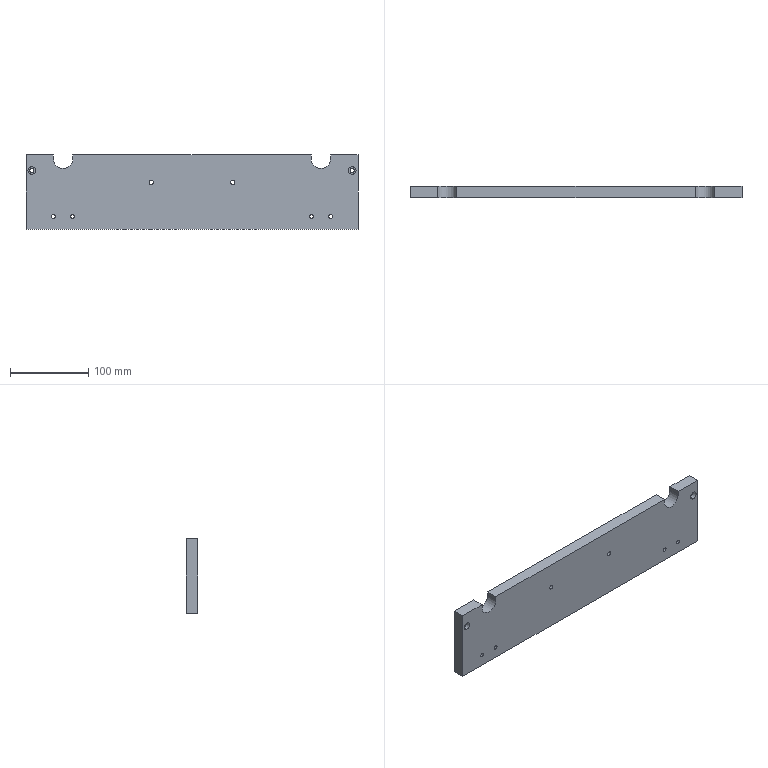Part | STEP file | Front side plate A | 1 solid | 56 faces | box 425 x 15 x 95 mm | volume 590562 mm3 | cylinder 32 | plane 14 | cone 10 | commonest cylinder face diameters 4.2 x10 5 x8 5.5 x8 10 x4 25 x2